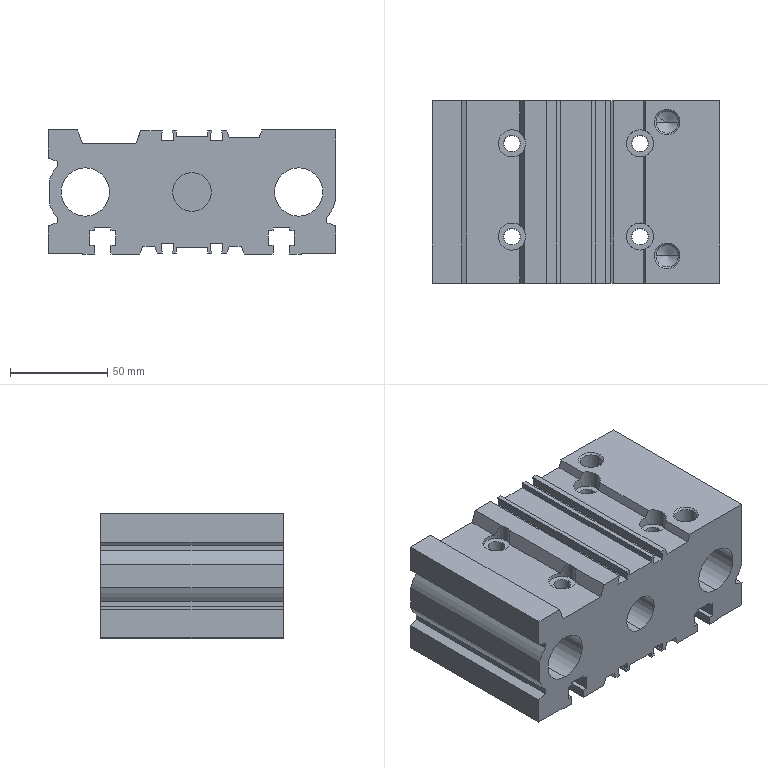Part | SolidWorks | features BaseBody 1 | 1 solid | 229 faces | box 148 x 94 x 64 mm | volume 563266 mm3 | plane 125 | cylinder 64 | cone 40 | commonest cylinder face diameters 8.376 x16 5 x13 8.6 x8 11.445 x8 14 x8 25 x4